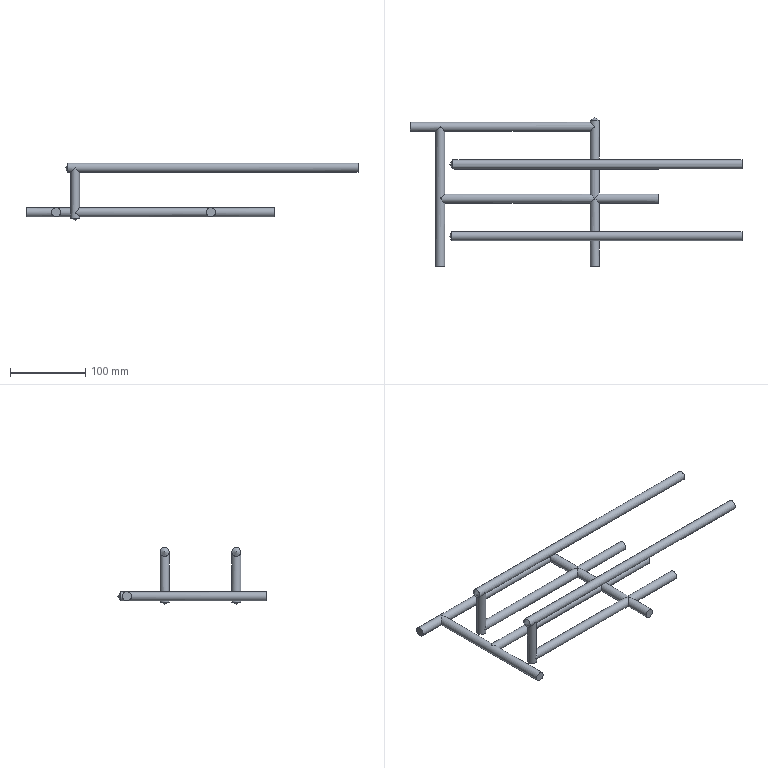Part | STEP file | SOLID | 1 solid | 29 faces | box 440 x 197.312 x 76 mm | volume 258377 mm3 | cylinder 16 | plane 8 | cone 5 | commonest cylinder face diameters 12 x16